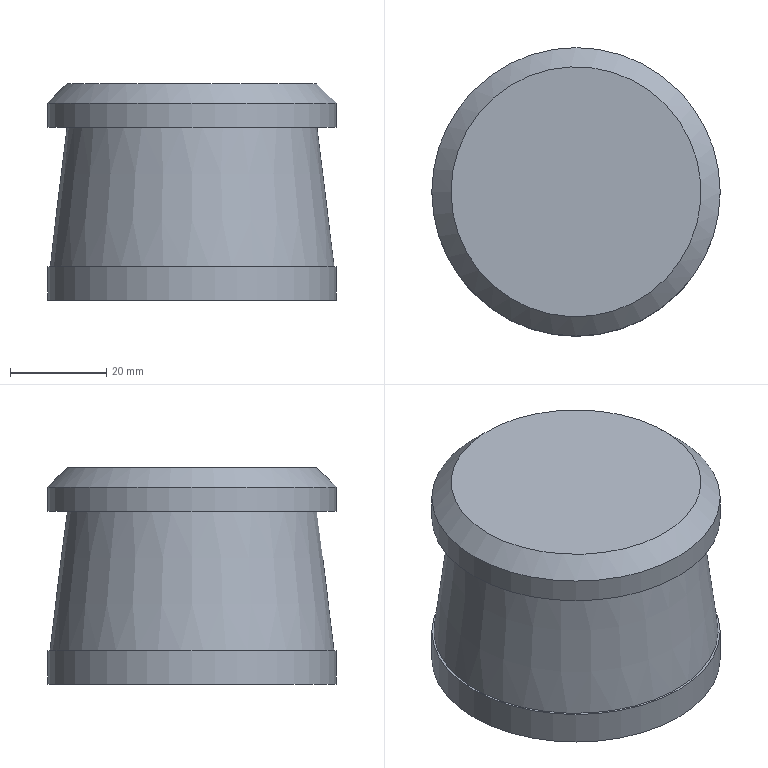Part | NX | features BREP 1 | 1 solid | 11 faces | box 60 x 60 x 45 mm | volume 73869 mm3 | plane 6 | cylinder 3 | cone 2 | commonest cylinder face diameters 60 x2 40 x1
STEP:
#1=CARTESIAN_POINT('',(30.,0.,-59.));
#2=VERTEX_POINT('',#1);
#3=CARTESIAN_POINT('',(0.,0.,-59.));
#4=DIRECTION('',(0.,0.,-1.));
#5=DIRECTION('',(1.,0.,0.));
#6=AXIS2_PLACEMENT_3D('',#3,#4,#5);
#7=CIRCLE('',#6,30.);
#8=EDGE_CURVE('',#2,#2,#7,.T.);
#9=ORIENTED_EDGE('',*,*,#8,.F.);
#10=EDGE_LOOP('',(#9));
#11=FACE_BOUND('',#10,.T.);
#12=CARTESIAN_POINT('',(30.,0.,-52.));
#13=VERTEX_POINT('',#12);
#14=CARTESIAN_POINT('',(0.,0.,-52.));
#15=DIRECTION('',(0.,0.,-1.));
#16=DIRECTION('',(1.,0.,0.));
#17=AXIS2_PLACEMENT_3D('',#14,#15,#16);
#18=CIRCLE('',#17,30.);
#19=EDGE_CURVE('',#13,#13,#18,.T.);
#20=ORIENTED_EDGE('',*,*,#19,.T.);
#21=EDGE_LOOP('',(#20));
#22=FACE_BOUND('',#21,.T.);
#23=CARTESIAN_POINT('',(0.,0.,-24.));
#24=DIRECTION('',(0.,0.,-1.));
#25=DIRECTION('',(1.,0.,0.));
#26=AXIS2_PLACEMENT_3D('',#23,#24,#25);
#27=CYLINDRICAL_SURFACE('',#26,30.);
#28=ADVANCED_FACE('',(#11,#22),#27,.T.);
#29=CARTESIAN_POINT('',(-13.775,-14.5,-59.));
#30=VERTEX_POINT('',#29);
#31=CARTESIAN_POINT('',(13.775,-14.5,-59.));
#32=VERTEX_POINT('',#31);
#33=CARTESIAN_POINT('',(0.,0.,-59.));
#34=DIRECTION('',(0.,0.,-1.));
#35=DIRECTION('',(0.766,0.6428,0.));
#36=AXIS2_PLACEMENT_3D('',#33,#34,#35);
#37=CIRCLE('',#36,20.);
#38=EDGE_CURVE('',#30,#32,#37,.T.);
#39=ORIENTED_EDGE('',*,*,#38,.T.);
#40=CARTESIAN_POINT('',(13.775,-14.5,-24.));
#41=VERTEX_POINT('',#40);
#42=CARTESIAN_POINT('',(13.775,-14.5,-24.));
#43=DIRECTION('',(0.,0.,1.));
#44=VECTOR('',#43,1000.);
#45=LINE('',#42,#44);
#46=EDGE_CURVE('',#32,#41,#45,.T.);
#47=ORIENTED_EDGE('',*,*,#46,.T.);
#48=CARTESIAN_POINT('',(-13.775,-14.5,-24.));
#49=VERTEX_POINT('',#48);
#50=CARTESIAN_POINT('',(0.,0.,-24.));
#51=DIRECTION('',(0.,0.,-1.));
#52=DIRECTION('',(0.766,0.6428,0.));
#53=AXIS2_PLACEMENT_3D('',#50,#51,#52);
#54=CIRCLE('',#53,20.);
#55=EDGE_CURVE('',#49,#41,#54,.T.);
#56=ORIENTED_EDGE('',*,*,#55,.F.);
#57=CARTESIAN_POINT('',(-13.775,-14.5,-24.));
#58=DIRECTION('',(0.,0.,-1.));
#59=VECTOR('',#58,1000.);
#60=LINE('',#57,#59);
#61=EDGE_CURVE('',#49,#30,#60,.T.);
#62=ORIENTED_EDGE('',*,*,#61,.T.);
#63=EDGE_LOOP('',(#39,#47,#56,#62));
#64=FACE_BOUND('',#63,.T.);
#65=CARTESIAN_POINT('',(0.,0.,-24.));
#66=DIRECTION('',(0.,0.,-1.));
#67=DIRECTION('',(1.,0.,0.));
#68=AXIS2_PLACEMENT_3D('',#65,#66,#67);
#69=CYLINDRICAL_SURFACE('',#68,20.);
#70=ADVANCED_FACE('',(#64),#69,.F.);
#71=CARTESIAN_POINT('',(13.775,-14.5,-59.));
#72=DIRECTION('',(-1.,0.,0.));
#73=VECTOR('',#72,1000.);
#74=LINE('',#71,#73);
#75=EDGE_CURVE('',#32,#30,#74,.T.);
#76=ORIENTED_EDGE('',*,*,#75,.T.);
#77=ORIENTED_EDGE('',*,*,#61,.F.);
#78=CARTESIAN_POINT('',(13.775,-14.5,-24.));
#79=DIRECTION('',(-1.,0.,0.));
#80=VECTOR('',#79,1000.);
#81=LINE('',#78,#80);
#82=EDGE_CURVE('',#41,#49,#81,.T.);
#83=ORIENTED_EDGE('',*,*,#82,.F.);
#84=ORIENTED_EDGE('',*,*,#46,.F.);
#85=EDGE_LOOP('',(#76,#77,#83,#84));
#86=FACE_BOUND('',#85,.T.);
#87=CARTESIAN_POINT('',(13.775,-14.5,-24.));
#88=DIRECTION('',(0.,-1.,0.));
#89=DIRECTION('',(0.,0.,1.));
#90=AXIS2_PLACEMENT_3D('',#87,#88,#89);
#91=PLANE('',#90);
#92=ADVANCED_FACE('',(#86),#91,.F.);
#93=ORIENTED_EDGE('',*,*,#8,.T.);
#94=EDGE_LOOP('',(#93));
#95=FACE_BOUND('',#94,.T.);
#96=ORIENTED_EDGE('',*,*,#38,.F.);
#97=ORIENTED_EDGE('',*,*,#75,.F.);
#98=EDGE_LOOP('',(#96,#97));
#99=FACE_BOUND('',#98,.T.);
#100=CARTESIAN_POINT('',(0.,0.,-59.));
#101=DIRECTION('',(0.,0.,-1.));
#102=DIRECTION('',(1.,0.,0.));
#103=AXIS2_PLACEMENT_3D('',#100,#101,#102);
#104=PLANE('',#103);
#105=ADVANCED_FACE('',(#95,#99),#104,.T.);
#106=ORIENTED_EDGE('',*,*,#82,.T.);
#107=ORIENTED_EDGE('',*,*,#55,.T.);
#108=EDGE_LOOP('',(#106,#107));
#109=FACE_BOUND('',#108,.T.);
#110=CARTESIAN_POINT('',(0.,0.,-24.));
#111=DIRECTION('',(0.,0.,-1.));
#112=DIRECTION('',(1.,0.,0.));
#113=AXIS2_PLACEMENT_3D('',#110,#111,#112);
#114=PLANE('',#113);
#115=ADVANCED_FACE('',(#109),#114,.T.);
#116=CARTESIAN_POINT('',(29.561,0.,-52.));
#117=VERTEX_POINT('',#116);
#118=CARTESIAN_POINT('',(0.,0.,-52.));
#119=DIRECTION('',(0.,0.,1.));
#120=DIRECTION('',(1.,0.,0.));
#121=AXIS2_PLACEMENT_3D('',#118,#119,#120);
#122=CIRCLE('',#121,29.561);
#123=EDGE_CURVE('',#117,#117,#122,.T.);
#124=ORIENTED_EDGE('',*,*,#123,.T.);
#125=EDGE_LOOP('',(#124));
#126=FACE_BOUND('',#125,.T.);
#127=CARTESIAN_POINT('',(-26.,0.,-23.));
#128=VERTEX_POINT('',#127);
#129=CARTESIAN_POINT('',(0.,0.,-23.));
#130=DIRECTION('',(0.,0.,1.));
#131=DIRECTION('',(-1.,0.,0.));
#132=AXIS2_PLACEMENT_3D('',#129,#130,#131);
#133=CIRCLE('',#132,26.);
#134=EDGE_CURVE('',#128,#128,#133,.T.);
#135=ORIENTED_EDGE('',*,*,#134,.F.);
#136=EDGE_LOOP('',(#135));
#137=FACE_BOUND('',#136,.T.);
#138=CARTESIAN_POINT('',(0.,0.,-23.));
#139=DIRECTION('',(0.,0.,-1.));
#140=DIRECTION('',(1.,0.,0.));
#141=AXIS2_PLACEMENT_3D('',#138,#139,#140);
#142=CONICAL_SURFACE('',#141,26.,0.1222);
#143=ADVANCED_FACE('',(#126,#137),#142,.T.);
#144=ORIENTED_EDGE('',*,*,#19,.F.);
#145=EDGE_LOOP('',(#144));
#146=FACE_BOUND('',#145,.T.);
#147=ORIENTED_EDGE('',*,*,#123,.F.);
#148=EDGE_LOOP('',(#147));
#149=FACE_BOUND('',#148,.T.);
#150=CARTESIAN_POINT('',(0.,0.,-52.));
#151=DIRECTION('',(0.,0.,1.));
#152=DIRECTION('',(-1.,0.,0.));
#153=AXIS2_PLACEMENT_3D('',#150,#151,#152);
#154=PLANE('',#153);
#155=ADVANCED_FACE('',(#146,#149),#154,.T.);
#156=CARTESIAN_POINT('',(30.,0.,-23.));
#157=VERTEX_POINT('',#156);
#158=CARTESIAN_POINT('',(0.,0.,-23.));
#159=DIRECTION('',(0.,0.,-1.));
#160=DIRECTION('',(1.,0.,0.));
#161=AXIS2_PLACEMENT_3D('',#158,#159,#160);
#162=CIRCLE('',#161,30.);
#163=EDGE_CURVE('',#157,#157,#162,.T.);
#164=ORIENTED_EDGE('',*,*,#163,.T.);
#165=EDGE_LOOP('',(#164));
#166=FACE_BOUND('',#165,.T.);
#167=ORIENTED_EDGE('',*,*,#134,.T.);
#168=EDGE_LOOP('',(#167));
#169=FACE_BOUND('',#168,.T.);
#170=CARTESIAN_POINT('',(0.,0.,-23.));
#171=DIRECTION('',(0.,0.,1.));
#172=DIRECTION('',(-1.,0.,0.));
#173=AXIS2_PLACEMENT_3D('',#170,#171,#172);
#174=PLANE('',#173);
#175=ADVANCED_FACE('',(#166,#169),#174,.F.);
#176=CARTESIAN_POINT('',(-26.,0.,-14.));
#177=VERTEX_POINT('',#176);
#178=CARTESIAN_POINT('',(0.,0.,-14.));
#179=DIRECTION('',(0.,0.,1.));
#180=DIRECTION('',(-1.,0.,0.));
#181=AXIS2_PLACEMENT_3D('',#178,#179,#180);
#182=CIRCLE('',#181,26.);
#183=EDGE_CURVE('',#177,#177,#182,.T.);
#184=ORIENTED_EDGE('',*,*,#183,.T.);
#185=EDGE_LOOP('',(#184));
#186=FACE_BOUND('',#185,.T.);
#187=CARTESIAN_POINT('',(0.,0.,-14.));
#188=DIRECTION('',(0.,0.,-1.));
#189=DIRECTION('',(1.,0.,0.));
#190=AXIS2_PLACEMENT_3D('',#187,#188,#189);
#191=PLANE('',#190);
#192=ADVANCED_FACE('',(#186),#191,.F.);
#193=ORIENTED_EDGE('',*,*,#183,.F.);
#194=EDGE_LOOP('',(#193));
#195=FACE_BOUND('',#194,.T.);
#196=CARTESIAN_POINT('',(-30.,0.,-18.));
#197=VERTEX_POINT('',#196);
#198=CARTESIAN_POINT('',(0.,0.,-18.));
#199=DIRECTION('',(0.,0.,-1.));
#200=DIRECTION('',(-1.,0.,0.));
#201=AXIS2_PLACEMENT_3D('',#198,#199,#200);
#202=CIRCLE('',#201,30.);
#203=EDGE_CURVE('',#197,#197,#202,.T.);
#204=ORIENTED_EDGE('',*,*,#203,.F.);
#205=EDGE_LOOP('',(#204));
#206=FACE_BOUND('',#205,.T.);
#207=CARTESIAN_POINT('',(0.,0.,-18.));
#208=DIRECTION('',(0.,0.,-1.));
#209=DIRECTION('',(1.,0.,0.));
#210=AXIS2_PLACEMENT_3D('',#207,#208,#209);
#211=CONICAL_SURFACE('',#210,30.,0.7854);
#212=ADVANCED_FACE('',(#195,#206),#211,.T.);
#213=ORIENTED_EDGE('',*,*,#163,.F.);
#214=EDGE_LOOP('',(#213));
#215=FACE_BOUND('',#214,.T.);
#216=ORIENTED_EDGE('',*,*,#203,.T.);
#217=EDGE_LOOP('',(#216));
#218=FACE_BOUND('',#217,.T.);
#219=CARTESIAN_POINT('',(0.,0.,-24.));
#220=DIRECTION('',(0.,0.,-1.));
#221=DIRECTION('',(1.,0.,0.));
#222=AXIS2_PLACEMENT_3D('',#219,#220,#221);
#223=CYLINDRICAL_SURFACE('',#222,30.);
#224=ADVANCED_FACE('',(#215,#218),#223,.T.);
#225=CLOSED_SHELL('',(#28,#70,#92,#105,#115,#143,#155,#175,#192,#212,#224));
#226=MANIFOLD_SOLID_BREP('',#225);
#227=(LENGTH_UNIT()NAMED_UNIT(*)SI_UNIT(.MILLI.,.METRE.));
#228=UNCERTAINTY_MEASURE_WITH_UNIT(LENGTH_MEASURE(0.00001),#227,'','');
#229=(NAMED_UNIT(*)PLANE_ANGLE_UNIT()SI_UNIT($,.RADIAN.));
#230=(NAMED_UNIT(*)SI_UNIT($,.STERADIAN.)SOLID_ANGLE_UNIT());
#231=(GEOMETRIC_REPRESENTATION_CONTEXT(3)GLOBAL_UNCERTAINTY_ASSIGNED_CONTEXT((#228))GLOBAL_UNIT_ASSIGNED_CONTEXT((#227,#229,#230))REPRESENTATION_CONTEXT('',''));
#232=ADVANCED_BREP_SHAPE_REPRESENTATION('',(#226),#231);